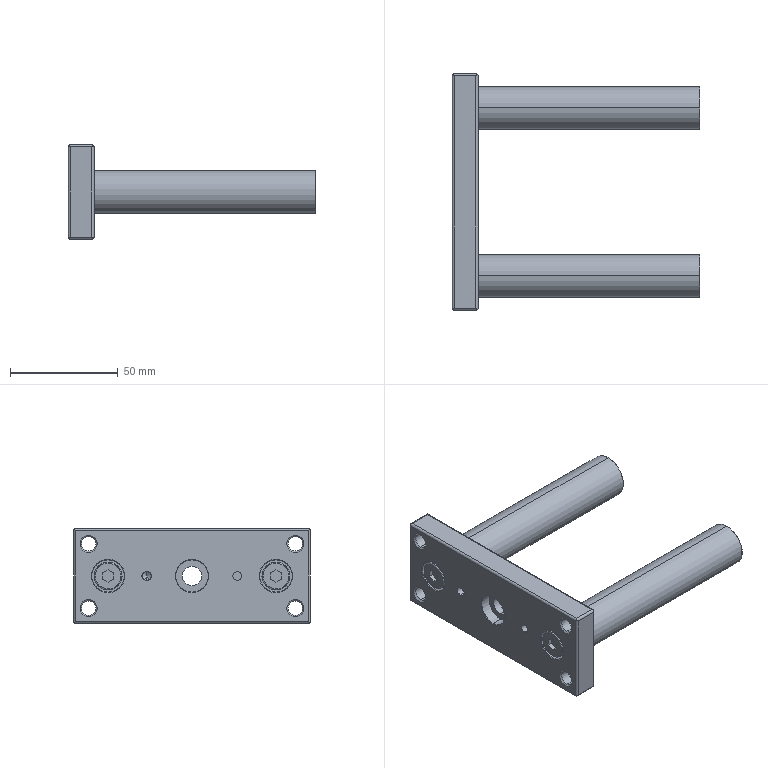Part | SolidWorks | features BaseBody 1 | 1 solid | 106 faces | box 115 x 110 x 44 mm | volume 118873 mm3 | cylinder 42 | plane 32 | cone 28 | spline 4 | commonest cylinder face diameters 2 x12 6.647 x8 4 x6 15 x6 13 x4 20 x4